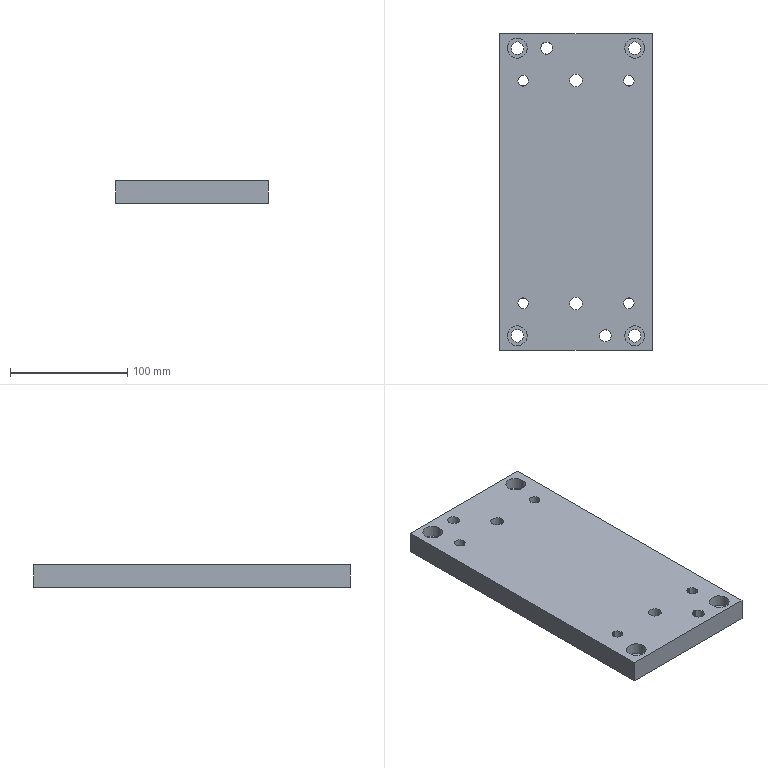Part | STEP file | YBQDJ-PD-6 | 1 solid | 52 faces | box 130 x 270 x 19 mm | volume 640127 mm3 | cylinder 36 | plane 12 | cone 4 | commonest cylinder face diameters 4 x12 1 x6 10.7 x6 17 x6 9 x4 10.01 x2